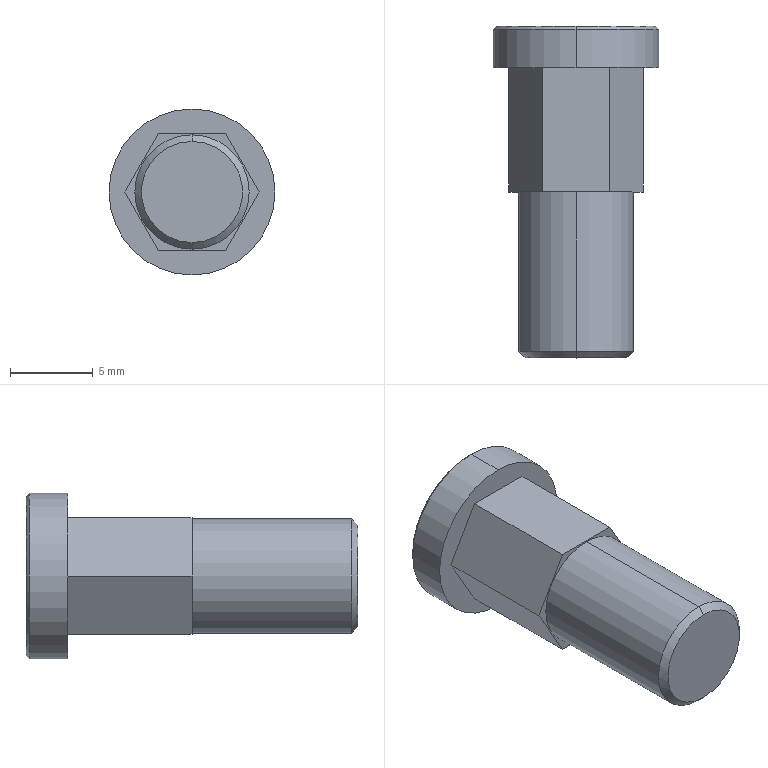Part | NX | features BREP 1 | 1 solid | 24 faces | box 10 x 20 x 10 mm | volume 454.713 mm3 | plane 12 | cylinder 8 | cone 4 | commonest cylinder face diameters 5 x2 6.2 x2 6.9 x2 10 x2
STEP:
#1=CARTESIAN_POINT('',(0.,-10.,-3.45));
#2=VERTEX_POINT('',#1);
#3=CARTESIAN_POINT('',(0.,-10.,3.45));
#4=VERTEX_POINT('',#3);
#5=CARTESIAN_POINT('',(0.,-10.,0.));
#6=DIRECTION('',(0.,-1.,0.));
#7=DIRECTION('',(0.,0.,-1.));
#8=AXIS2_PLACEMENT_3D('',#5,#6,#7);
#9=CIRCLE('',#8,3.45);
#10=EDGE_CURVE('',#2,#4,#9,.T.);
#11=ORIENTED_EDGE('',*,*,#10,.T.);
#12=CARTESIAN_POINT('',(0.,-19.6,3.45));
#13=VERTEX_POINT('',#12);
#14=CARTESIAN_POINT('',(0.,-20.,3.45));
#15=DIRECTION('',(0.,-1.,0.));
#16=VECTOR('',#15,1000.);
#17=LINE('',#14,#16);
#18=EDGE_CURVE('',#13,#4,#17,.F.);
#19=ORIENTED_EDGE('',*,*,#18,.F.);
#20=CARTESIAN_POINT('',(0.,-19.6,-3.45));
#21=VERTEX_POINT('',#20);
#22=CARTESIAN_POINT('',(0.,-19.6,0.));
#23=DIRECTION('',(0.,1.,0.));
#24=DIRECTION('',(0.,0.,-1.));
#25=AXIS2_PLACEMENT_3D('',#22,#23,#24);
#26=CIRCLE('',#25,3.45);
#27=EDGE_CURVE('',#13,#21,#26,.T.);
#28=ORIENTED_EDGE('',*,*,#27,.T.);
#29=CARTESIAN_POINT('',(0.,-20.,-3.45));
#30=DIRECTION('',(0.,-1.,0.));
#31=VECTOR('',#30,1000.);
#32=LINE('',#29,#31);
#33=EDGE_CURVE('',#21,#2,#32,.F.);
#34=ORIENTED_EDGE('',*,*,#33,.T.);
#35=EDGE_LOOP('',(#11,#19,#28,#34));
#36=FACE_BOUND('',#35,.T.);
#37=CARTESIAN_POINT('',(0.,-20.,0.));
#38=DIRECTION('',(0.,-1.,0.));
#39=DIRECTION('',(0.,0.,1.));
#40=AXIS2_PLACEMENT_3D('',#37,#38,#39);
#41=CYLINDRICAL_SURFACE('',#40,3.45);
#42=ADVANCED_FACE('',(#36),#41,.T.);
#43=CARTESIAN_POINT('',(0.,-20.,3.05));
#44=VERTEX_POINT('',#43);
#45=CARTESIAN_POINT('',(0.,-20.,-3.05));
#46=VERTEX_POINT('',#45);
#47=CARTESIAN_POINT('',(0.,-20.,0.));
#48=DIRECTION('',(0.,1.,0.));
#49=DIRECTION('',(0.,0.,1.));
#50=AXIS2_PLACEMENT_3D('',#47,#48,#49);
#51=CIRCLE('',#50,3.05);
#52=EDGE_CURVE('',#44,#46,#51,.T.);
#53=ORIENTED_EDGE('',*,*,#52,.T.);
#54=CARTESIAN_POINT('',(0.,-19.6,-3.45));
#55=DIRECTION('',(0.,0.7071,-0.7071));
#56=VECTOR('',#55,1000.);
#57=LINE('',#54,#56);
#58=EDGE_CURVE('',#46,#21,#57,.T.);
#59=ORIENTED_EDGE('',*,*,#58,.T.);
#60=ORIENTED_EDGE('',*,*,#27,.F.);
#61=CARTESIAN_POINT('',(0.,-19.6,3.45));
#62=DIRECTION('',(0.,0.7071,0.7071));
#63=VECTOR('',#62,1000.);
#64=LINE('',#61,#63);
#65=EDGE_CURVE('',#44,#13,#64,.T.);
#66=ORIENTED_EDGE('',*,*,#65,.F.);
#67=EDGE_LOOP('',(#53,#59,#60,#66));
#68=FACE_BOUND('',#67,.T.);
#69=CARTESIAN_POINT('',(0.,-19.6,0.));
#70=DIRECTION('',(0.,1.,0.));
#71=DIRECTION('',(0.,0.,-1.));
#72=AXIS2_PLACEMENT_3D('',#69,#70,#71);
#73=CONICAL_SURFACE('',#72,3.45,0.7854);
#74=ADVANCED_FACE('',(#68),#73,.T.);
#75=CARTESIAN_POINT('',(0.,-2.5,5.));
#76=VERTEX_POINT('',#75);
#77=CARTESIAN_POINT('',(0.,-2.5,-5.));
#78=VERTEX_POINT('',#77);
#79=CARTESIAN_POINT('',(0.,-2.5,0.));
#80=DIRECTION('',(0.,1.,0.));
#81=DIRECTION('',(0.,0.,1.));
#82=AXIS2_PLACEMENT_3D('',#79,#80,#81);
#83=CIRCLE('',#82,5.);
#84=EDGE_CURVE('',#76,#78,#83,.T.);
#85=ORIENTED_EDGE('',*,*,#84,.T.);
#86=CARTESIAN_POINT('',(0.,-0.2,-5.));
#87=VERTEX_POINT('',#86);
#88=CARTESIAN_POINT('',(0.,0.,-5.));
#89=DIRECTION('',(0.,1.,0.));
#90=VECTOR('',#89,1000.);
#91=LINE('',#88,#90);
#92=EDGE_CURVE('',#78,#87,#91,.T.);
#93=ORIENTED_EDGE('',*,*,#92,.T.);
#94=CARTESIAN_POINT('',(0.,-0.2,5.));
#95=VERTEX_POINT('',#94);
#96=CARTESIAN_POINT('',(0.,-0.2,0.));
#97=DIRECTION('',(0.,-1.,0.));
#98=DIRECTION('',(0.,0.,1.));
#99=AXIS2_PLACEMENT_3D('',#96,#97,#98);
#100=CIRCLE('',#99,5.);
#101=EDGE_CURVE('',#87,#95,#100,.T.);
#102=ORIENTED_EDGE('',*,*,#101,.T.);
#103=CARTESIAN_POINT('',(0.,0.,5.));
#104=DIRECTION('',(0.,1.,0.));
#105=VECTOR('',#104,1000.);
#106=LINE('',#103,#105);
#107=EDGE_CURVE('',#76,#95,#106,.T.);
#108=ORIENTED_EDGE('',*,*,#107,.F.);
#109=EDGE_LOOP('',(#85,#93,#102,#108));
#110=FACE_BOUND('',#109,.T.);
#111=CARTESIAN_POINT('',(0.,0.,0.));
#112=DIRECTION('',(0.,1.,0.));
#113=DIRECTION('',(0.,0.,-1.));
#114=AXIS2_PLACEMENT_3D('',#111,#112,#113);
#115=CYLINDRICAL_SURFACE('',#114,5.);
#116=ADVANCED_FACE('',(#110),#115,.T.);
#117=CARTESIAN_POINT('',(0.,0.,-4.8));
#118=VERTEX_POINT('',#117);
#119=CARTESIAN_POINT('',(0.,0.,4.8));
#120=VERTEX_POINT('',#119);
#121=CARTESIAN_POINT('',(0.,0.,0.));
#122=DIRECTION('',(0.,-1.,0.));
#123=DIRECTION('',(0.,0.,-1.));
#124=AXIS2_PLACEMENT_3D('',#121,#122,#123);
#125=CIRCLE('',#124,4.8);
#126=EDGE_CURVE('',#118,#120,#125,.T.);
#127=ORIENTED_EDGE('',*,*,#126,.T.);
#128=CARTESIAN_POINT('',(0.,-0.2,5.));
#129=DIRECTION('',(0.,-0.7071,0.7071));
#130=VECTOR('',#129,1000.);
#131=LINE('',#128,#130);
#132=EDGE_CURVE('',#95,#120,#131,.F.);
#133=ORIENTED_EDGE('',*,*,#132,.F.);
#134=ORIENTED_EDGE('',*,*,#101,.F.);
#135=CARTESIAN_POINT('',(0.,-0.2,-5.));
#136=DIRECTION('',(0.,-0.7071,-0.7071));
#137=VECTOR('',#136,1000.);
#138=LINE('',#135,#137);
#139=EDGE_CURVE('',#87,#118,#138,.F.);
#140=ORIENTED_EDGE('',*,*,#139,.T.);
#141=EDGE_LOOP('',(#127,#133,#134,#140));
#142=FACE_BOUND('',#141,.T.);
#143=CARTESIAN_POINT('',(0.,-0.2,0.));
#144=DIRECTION('',(0.,-1.,0.));
#145=DIRECTION('',(0.,0.,1.));
#146=AXIS2_PLACEMENT_3D('',#143,#144,#145);
#147=CONICAL_SURFACE('',#146,5.,0.7854);
#148=ADVANCED_FACE('',(#142),#147,.T.);
#149=CARTESIAN_POINT('',(0.,-7.4,-3.1));
#150=VERTEX_POINT('',#149);
#151=CARTESIAN_POINT('',(0.,-7.4,3.1));
#152=VERTEX_POINT('',#151);
#153=CARTESIAN_POINT('',(0.,-7.4,0.));
#154=DIRECTION('',(0.,1.,0.));
#155=DIRECTION('',(0.,0.,1.));
#156=AXIS2_PLACEMENT_3D('',#153,#154,#155);
#157=CIRCLE('',#156,3.1);
#158=EDGE_CURVE('',#150,#152,#157,.T.);
#159=ORIENTED_EDGE('',*,*,#158,.F.);
#160=CARTESIAN_POINT('',(0.,0.,-3.1));
#161=VERTEX_POINT('',#160);
#162=CARTESIAN_POINT('',(0.,0.,-3.1));
#163=DIRECTION('',(0.,1.,0.));
#164=VECTOR('',#163,1000.);
#165=LINE('',#162,#164);
#166=EDGE_CURVE('',#150,#161,#165,.T.);
#167=ORIENTED_EDGE('',*,*,#166,.T.);
#168=CARTESIAN_POINT('',(0.,0.,3.1));
#169=VERTEX_POINT('',#168);
#170=CARTESIAN_POINT('',(0.,0.,0.));
#171=DIRECTION('',(0.,-1.,0.));
#172=DIRECTION('',(0.,0.,1.));
#173=AXIS2_PLACEMENT_3D('',#170,#171,#172);
#174=CIRCLE('',#173,3.1);
#175=EDGE_CURVE('',#169,#161,#174,.T.);
#176=ORIENTED_EDGE('',*,*,#175,.F.);
#177=CARTESIAN_POINT('',(0.,0.,3.1));
#178=DIRECTION('',(0.,1.,0.));
#179=VECTOR('',#178,1000.);
#180=LINE('',#177,#179);
#181=EDGE_CURVE('',#152,#169,#180,.T.);
#182=ORIENTED_EDGE('',*,*,#181,.F.);
#183=EDGE_LOOP('',(#159,#167,#176,#182));
#184=FACE_BOUND('',#183,.T.);
#185=CARTESIAN_POINT('',(0.,0.,0.));
#186=DIRECTION('',(0.,1.,0.));
#187=DIRECTION('',(0.,0.,-1.));
#188=AXIS2_PLACEMENT_3D('',#185,#186,#187);
#189=CYLINDRICAL_SURFACE('',#188,3.1);
#190=ADVANCED_FACE('',(#184),#189,.F.);
#191=CARTESIAN_POINT('',(0.,-18.,-2.5));
#192=VERTEX_POINT('',#191);
#193=CARTESIAN_POINT('',(0.,-18.,2.5));
#194=VERTEX_POINT('',#193);
#195=CARTESIAN_POINT('',(0.,-18.,0.));
#196=DIRECTION('',(0.,1.,0.));
#197=DIRECTION('',(0.,0.,1.));
#198=AXIS2_PLACEMENT_3D('',#195,#196,#197);
#199=CIRCLE('',#198,2.5);
#200=EDGE_CURVE('',#192,#194,#199,.T.);
#201=ORIENTED_EDGE('',*,*,#200,.F.);
#202=CARTESIAN_POINT('',(0.,-7.4,-2.5));
#203=VERTEX_POINT('',#202);
#204=CARTESIAN_POINT('',(0.,-7.4,-2.5));
#205=DIRECTION('',(0.,1.,0.));
#206=VECTOR('',#205,1000.);
#207=LINE('',#204,#206);
#208=EDGE_CURVE('',#192,#203,#207,.T.);
#209=ORIENTED_EDGE('',*,*,#208,.T.);
#210=CARTESIAN_POINT('',(0.,-7.4,2.5));
#211=VERTEX_POINT('',#210);
#212=CARTESIAN_POINT('',(0.,-7.4,0.));
#213=DIRECTION('',(0.,-1.,0.));
#214=DIRECTION('',(0.,0.,1.));
#215=AXIS2_PLACEMENT_3D('',#212,#213,#214);
#216=CIRCLE('',#215,2.5);
#217=EDGE_CURVE('',#211,#203,#216,.T.);
#218=ORIENTED_EDGE('',*,*,#217,.F.);
#219=CARTESIAN_POINT('',(0.,-7.4,2.5));
#220=DIRECTION('',(0.,1.,0.));
#221=VECTOR('',#220,1000.);
#222=LINE('',#219,#221);
#223=EDGE_CURVE('',#194,#211,#222,.T.);
#224=ORIENTED_EDGE('',*,*,#223,.F.);
#225=EDGE_LOOP('',(#201,#209,#218,#224));
#226=FACE_BOUND('',#225,.T.);
#227=CARTESIAN_POINT('',(0.,-7.4,0.));
#228=DIRECTION('',(0.,1.,0.));
#229=DIRECTION('',(0.,0.,-1.));
#230=AXIS2_PLACEMENT_3D('',#227,#228,#229);
#231=CYLINDRICAL_SURFACE('',#230,2.5);
#232=ADVANCED_FACE('',(#226),#231,.F.);
#233=ORIENTED_EDGE('',*,*,#18,.T.);
#234=CARTESIAN_POINT('',(0.,-10.,0.));
#235=DIRECTION('',(0.,-1.,0.));
#236=DIRECTION('',(0.,0.,-1.));
#237=AXIS2_PLACEMENT_3D('',#234,#235,#236);
#238=CIRCLE('',#237,3.45);
#239=EDGE_CURVE('',#4,#2,#238,.T.);
#240=ORIENTED_EDGE('',*,*,#239,.T.);
#241=ORIENTED_EDGE('',*,*,#33,.F.);
#242=CARTESIAN_POINT('',(0.,-19.6,0.));
#243=DIRECTION('',(0.,1.,0.));
#244=DIRECTION('',(0.,0.,-1.));
#245=AXIS2_PLACEMENT_3D('',#242,#243,#244);
#246=CIRCLE('',#245,3.45);
#247=EDGE_CURVE('',#21,#13,#246,.T.);
#248=ORIENTED_EDGE('',*,*,#247,.T.);
#249=EDGE_LOOP('',(#233,#240,#241,#248));
#250=FACE_BOUND('',#249,.T.);
#251=CARTESIAN_POINT('',(0.,-20.,0.));
#252=DIRECTION('',(0.,-1.,0.));
#253=DIRECTION('',(0.,0.,1.));
#254=AXIS2_PLACEMENT_3D('',#251,#252,#253);
#255=CYLINDRICAL_SURFACE('',#254,3.45);
#256=ADVANCED_FACE('',(#250),#255,.T.);
#257=ORIENTED_EDGE('',*,*,#58,.F.);
#258=CARTESIAN_POINT('',(0.,-20.,0.));
#259=DIRECTION('',(0.,1.,0.));
#260=DIRECTION('',(0.,0.,1.));
#261=AXIS2_PLACEMENT_3D('',#258,#259,#260);
#262=CIRCLE('',#261,3.05);
#263=EDGE_CURVE('',#46,#44,#262,.T.);
#264=ORIENTED_EDGE('',*,*,#263,.T.);
#265=ORIENTED_EDGE('',*,*,#65,.T.);
#266=ORIENTED_EDGE('',*,*,#247,.F.);
#267=EDGE_LOOP('',(#257,#264,#265,#266));
#268=FACE_BOUND('',#267,.T.);
#269=CARTESIAN_POINT('',(0.,-19.6,0.));
#270=DIRECTION('',(0.,1.,0.));
#271=DIRECTION('',(0.,0.,-1.));
#272=AXIS2_PLACEMENT_3D('',#269,#270,#271);
#273=CONICAL_SURFACE('',#272,3.45,0.7854);
#274=ADVANCED_FACE('',(#268),#273,.T.);
#275=CARTESIAN_POINT('',(-2.021,-10.,-3.5));
#276=VERTEX_POINT('',#275);
#277=CARTESIAN_POINT('',(2.021,-10.,-3.5));
#278=VERTEX_POINT('',#277);
#279=CARTESIAN_POINT('',(0.,-10.,-3.5));
#280=DIRECTION('',(1.,0.,0.));
#281=VECTOR('',#280,1000.);
#282=LINE('',#279,#281);
#283=EDGE_CURVE('',#276,#278,#282,.T.);
#284=ORIENTED_EDGE('',*,*,#283,.T.);
#285=CARTESIAN_POINT('',(4.041,-10.,0.));
#286=VERTEX_POINT('',#285);
#287=CARTESIAN_POINT('',(2.021,-10.,-3.5));
#288=DIRECTION('',(0.5,0.,0.866));
#289=VECTOR('',#288,1000.);
#290=LINE('',#287,#289);
#291=EDGE_CURVE('',#278,#286,#290,.T.);
#292=ORIENTED_EDGE('',*,*,#291,.T.);
#293=CARTESIAN_POINT('',(2.021,-10.,3.5));
#294=VERTEX_POINT('',#293);
#295=CARTESIAN_POINT('',(4.041,-10.,0.));
#296=DIRECTION('',(-0.5,0.,0.866));
#297=VECTOR('',#296,1000.);
#298=LINE('',#295,#297);
#299=EDGE_CURVE('',#286,#294,#298,.T.);
#300=ORIENTED_EDGE('',*,*,#299,.T.);
#301=CARTESIAN_POINT('',(-2.021,-10.,3.5));
#302=VERTEX_POINT('',#301);
#303=CARTESIAN_POINT('',(0.,-10.,3.5));
#304=DIRECTION('',(-1.,0.,0.));
#305=VECTOR('',#304,1000.);
#306=LINE('',#303,#305);
#307=EDGE_CURVE('',#294,#302,#306,.T.);
#308=ORIENTED_EDGE('',*,*,#307,.T.);
#309=CARTESIAN_POINT('',(-4.041,-10.,0.));
#310=VERTEX_POINT('',#309);
#311=CARTESIAN_POINT('',(-2.021,-10.,3.5));
#312=DIRECTION('',(-0.5,0.,-0.866));
#313=VECTOR('',#312,1000.);
#314=LINE('',#311,#313);
#315=EDGE_CURVE('',#302,#310,#314,.T.);
#316=ORIENTED_EDGE('',*,*,#315,.T.);
#317=CARTESIAN_POINT('',(-4.041,-10.,0.));
#318=DIRECTION('',(0.5,0.,-0.866));
#319=VECTOR('',#318,1000.);
#320=LINE('',#317,#319);
#321=EDGE_CURVE('',#310,#276,#320,.T.);
#322=ORIENTED_EDGE('',*,*,#321,.T.);
#323=EDGE_LOOP('',(#284,#292,#300,#308,#316,#322));
#324=FACE_BOUND('',#323,.T.);
#325=ORIENTED_EDGE('',*,*,#10,.F.);
#326=ORIENTED_EDGE('',*,*,#239,.F.);
#327=EDGE_LOOP('',(#325,#326));
#328=FACE_BOUND('',#327,.T.);
#329=CARTESIAN_POINT('',(0.,-10.,0.));
#330=DIRECTION('',(0.,-1.,0.));
#331=DIRECTION('',(0.,0.,1.));
#332=AXIS2_PLACEMENT_3D('',#329,#330,#331);
#333=PLANE('',#332);
#334=ADVANCED_FACE('',(#324,#328),#333,.T.);
#335=ORIENTED_EDGE('',*,*,#52,.F.);
#336=ORIENTED_EDGE('',*,*,#263,.F.);
#337=EDGE_LOOP('',(#335,#336));
#338=FACE_BOUND('',#337,.T.);
#339=CARTESIAN_POINT('',(0.,-20.,0.));
#340=DIRECTION('',(0.,-1.,0.));
#341=DIRECTION('',(0.,0.,1.));
#342=AXIS2_PLACEMENT_3D('',#339,#340,#341);
#343=PLANE('',#342);
#344=ADVANCED_FACE('',(#338),#343,.T.);
#345=CARTESIAN_POINT('',(2.021,-2.5,-3.5));
#346=VERTEX_POINT('',#345);
#347=CARTESIAN_POINT('',(2.021,-2.5,-3.5));
#348=DIRECTION('',(0.,1.,0.));
#349=VECTOR('',#348,1000.);
#350=LINE('',#347,#349);
#351=EDGE_CURVE('',#278,#346,#350,.T.);
#352=ORIENTED_EDGE('',*,*,#351,.T.);
#353=CARTESIAN_POINT('',(4.041,-2.5,0.));
#354=VERTEX_POINT('',#353);
#355=CARTESIAN_POINT('',(2.021,-2.5,-3.5));
#356=DIRECTION('',(0.5,0.,0.866));
#357=VECTOR('',#356,1000.);
#358=LINE('',#355,#357);
#359=EDGE_CURVE('',#346,#354,#358,.T.);
#360=ORIENTED_EDGE('',*,*,#359,.T.);
#361=CARTESIAN_POINT('',(4.041,-2.5,0.));
#362=DIRECTION('',(0.,-1.,0.));
#363=VECTOR('',#362,1000.);
#364=LINE('',#361,#363);
#365=EDGE_CURVE('',#354,#286,#364,.T.);
#366=ORIENTED_EDGE('',*,*,#365,.T.);
#367=ORIENTED_EDGE('',*,*,#291,.F.);
#368=EDGE_LOOP('',(#352,#360,#366,#367));
#369=FACE_BOUND('',#368,.T.);
#370=CARTESIAN_POINT('',(2.021,-2.5,-3.5));
#371=DIRECTION('',(0.866,0.,-0.5));
#372=DIRECTION('',(0.5,0.,0.866));
#373=AXIS2_PLACEMENT_3D('',#370,#371,#372);
#374=PLANE('',#373);
#375=ADVANCED_FACE('',(#369),#374,.T.);
#376=CARTESIAN_POINT('',(-2.021,-2.5,-3.5));
#377=VERTEX_POINT('',#376);
#378=CARTESIAN_POINT('',(-2.021,-2.5,-3.5));
#379=DIRECTION('',(0.,1.,0.));
#380=VECTOR('',#379,1000.);
#381=LINE('',#378,#380);
#382=EDGE_CURVE('',#276,#377,#381,.T.);
#383=ORIENTED_EDGE('',*,*,#382,.T.);
#384=CARTESIAN_POINT('',(-2.021,-2.5,-3.5));
#385=DIRECTION('',(1.,0.,0.));
#386=VECTOR('',#385,1000.);
#387=LINE('',#384,#386);
#388=EDGE_CURVE('',#377,#346,#387,.T.);
#389=ORIENTED_EDGE('',*,*,#388,.T.);
#390=ORIENTED_EDGE('',*,*,#351,.F.);
#391=ORIENTED_EDGE('',*,*,#283,.F.);
#392=EDGE_LOOP('',(#383,#389,#390,#391));
#393=FACE_BOUND('',#392,.T.);
#394=CARTESIAN_POINT('',(-2.021,-2.5,-3.5));
#395=DIRECTION('',(0.,0.,-1.));
#396=DIRECTION('',(1.,0.,0.));
#397=AXIS2_PLACEMENT_3D('',#394,#395,#396);
#398=PLANE('',#397);
#399=ADVANCED_FACE('',(#393),#398,.T.);
#400=CARTESIAN_POINT('',(-4.041,-2.5,0.));
#401=VERTEX_POINT('',#400);
#402=CARTESIAN_POINT('',(-4.041,-2.5,0.));
#403=DIRECTION('',(0.,1.,0.));
#404=VECTOR('',#403,1000.);
#405=LINE('',#402,#404);
#406=EDGE_CURVE('',#310,#401,#405,.T.);
#407=ORIENTED_EDGE('',*,*,#406,.T.);
#408=CARTESIAN_POINT('',(-4.041,-2.5,0.));
#409=DIRECTION('',(0.5,0.,-0.866));
#410=VECTOR('',#409,1000.);
#411=LINE('',#408,#410);
#412=EDGE_CURVE('',#401,#377,#411,.T.);
#413=ORIENTED_EDGE('',*,*,#412,.T.);
#414=ORIENTED_EDGE('',*,*,#382,.F.);
#415=ORIENTED_EDGE('',*,*,#321,.F.);
#416=EDGE_LOOP('',(#407,#413,#414,#415));
#417=FACE_BOUND('',#416,.T.);
#418=CARTESIAN_POINT('',(-4.041,-2.5,0.));
#419=DIRECTION('',(-0.866,0.,-0.5));
#420=DIRECTION('',(0.5,0.,-0.866));
#421=AXIS2_PLACEMENT_3D('',#418,#419,#420);
#422=PLANE('',#421);
#423=ADVANCED_FACE('',(#417),#422,.T.);
#424=CARTESIAN_POINT('',(-2.021,-2.5,3.5));
#425=VERTEX_POINT('',#424);
#426=CARTESIAN_POINT('',(-2.021,-2.5,3.5));
#427=DIRECTION('',(0.,1.,0.));
#428=VECTOR('',#427,1000.);
#429=LINE('',#426,#428);
#430=EDGE_CURVE('',#302,#425,#429,.T.);
#431=ORIENTED_EDGE('',*,*,#430,.T.);
#432=CARTESIAN_POINT('',(-2.021,-2.5,3.5));
#433=DIRECTION('',(-0.5,0.,-0.866));
#434=VECTOR('',#433,1000.);
#435=LINE('',#432,#434);
#436=EDGE_CURVE('',#425,#401,#435,.T.);
#437=ORIENTED_EDGE('',*,*,#436,.T.);
#438=ORIENTED_EDGE('',*,*,#406,.F.);
#439=ORIENTED_EDGE('',*,*,#315,.F.);
#440=EDGE_LOOP('',(#431,#437,#438,#439));
#441=FACE_BOUND('',#440,.T.);
#442=CARTESIAN_POINT('',(-2.021,-2.5,3.5));
#443=DIRECTION('',(-0.866,0.,0.5));
#444=DIRECTION('',(-0.5,0.,-0.866));
#445=AXIS2_PLACEMENT_3D('',#442,#443,#444);
#446=PLANE('',#445);
#447=ADVANCED_FACE('',(#441),#446,.T.);
#448=CARTESIAN_POINT('',(2.021,-2.5,3.5));
#449=VERTEX_POINT('',#448);
#450=CARTESIAN_POINT('',(2.021,-2.5,3.5));
#451=DIRECTION('',(0.,1.,0.));
#452=VECTOR('',#451,1000.);
#453=LINE('',#450,#452);
#454=EDGE_CURVE('',#294,#449,#453,.T.);
#455=ORIENTED_EDGE('',*,*,#454,.T.);
#456=CARTESIAN_POINT('',(2.021,-2.5,3.5));
#457=DIRECTION('',(-1.,0.,0.));
#458=VECTOR('',#457,1000.);
#459=LINE('',#456,#458);
#460=EDGE_CURVE('',#449,#425,#459,.T.);
#461=ORIENTED_EDGE('',*,*,#460,.T.);
#462=ORIENTED_EDGE('',*,*,#430,.F.);
#463=ORIENTED_EDGE('',*,*,#307,.F.);
#464=EDGE_LOOP('',(#455,#461,#462,#463));
#465=FACE_BOUND('',#464,.T.);
#466=CARTESIAN_POINT('',(2.021,-2.5,3.5));
#467=DIRECTION('',(0.,0.,1.));
#468=DIRECTION('',(-1.,0.,0.));
#469=AXIS2_PLACEMENT_3D('',#466,#467,#468);
#470=PLANE('',#469);
#471=ADVANCED_FACE('',(#465),#470,.T.);
#472=ORIENTED_EDGE('',*,*,#365,.F.);
#473=CARTESIAN_POINT('',(4.041,-2.5,0.));
#474=DIRECTION('',(-0.5,0.,0.866));
#475=VECTOR('',#474,1000.);
#476=LINE('',#473,#475);
#477=EDGE_CURVE('',#354,#449,#476,.T.);
#478=ORIENTED_EDGE('',*,*,#477,.T.);
#479=ORIENTED_EDGE('',*,*,#454,.F.);
#480=ORIENTED_EDGE('',*,*,#299,.F.);
#481=EDGE_LOOP('',(#472,#478,#479,#480));
#482=FACE_BOUND('',#481,.T.);
#483=CARTESIAN_POINT('',(4.041,-2.5,0.));
#484=DIRECTION('',(0.866,0.,0.5));
#485=DIRECTION('',(-0.5,0.,0.866));
#486=AXIS2_PLACEMENT_3D('',#483,#484,#485);
#487=PLANE('',#486);
#488=ADVANCED_FACE('',(#482),#487,.T.);
#489=ORIENTED_EDGE('',*,*,#84,.F.);
#490=CARTESIAN_POINT('',(0.,-2.5,0.));
#491=DIRECTION('',(0.,1.,0.));
#492=DIRECTION('',(0.,0.,1.));
#493=AXIS2_PLACEMENT_3D('',#490,#491,#492);
#494=CIRCLE('',#493,5.);
#495=EDGE_CURVE('',#78,#76,#494,.T.);
#496=ORIENTED_EDGE('',*,*,#495,.F.);
#497=EDGE_LOOP('',(#489,#496));
#498=FACE_BOUND('',#497,.T.);
#499=ORIENTED_EDGE('',*,*,#388,.F.);
#500=ORIENTED_EDGE('',*,*,#412,.F.);
#501=ORIENTED_EDGE('',*,*,#436,.F.);
#502=ORIENTED_EDGE('',*,*,#460,.F.);
#503=ORIENTED_EDGE('',*,*,#477,.F.);
#504=ORIENTED_EDGE('',*,*,#359,.F.);
#505=EDGE_LOOP('',(#499,#500,#501,#502,#503,#504));
#506=FACE_BOUND('',#505,.T.);
#507=CARTESIAN_POINT('',(0.,-2.5,0.));
#508=DIRECTION('',(0.,1.,0.));
#509=DIRECTION('',(0.,0.,-1.));
#510=AXIS2_PLACEMENT_3D('',#507,#508,#509);
#511=PLANE('',#510);
#512=ADVANCED_FACE('',(#498,#506),#511,.F.);
#513=ORIENTED_EDGE('',*,*,#92,.F.);
#514=ORIENTED_EDGE('',*,*,#495,.T.);
#515=ORIENTED_EDGE('',*,*,#107,.T.);
#516=CARTESIAN_POINT('',(0.,-0.2,0.));
#517=DIRECTION('',(0.,-1.,0.));
#518=DIRECTION('',(0.,0.,1.));
#519=AXIS2_PLACEMENT_3D('',#516,#517,#518);
#520=CIRCLE('',#519,5.);
#521=EDGE_CURVE('',#95,#87,#520,.T.);
#522=ORIENTED_EDGE('',*,*,#521,.T.);
#523=EDGE_LOOP('',(#513,#514,#515,#522));
#524=FACE_BOUND('',#523,.T.);
#525=CARTESIAN_POINT('',(0.,0.,0.));
#526=DIRECTION('',(0.,1.,0.));
#527=DIRECTION('',(0.,0.,-1.));
#528=AXIS2_PLACEMENT_3D('',#525,#526,#527);
#529=CYLINDRICAL_SURFACE('',#528,5.);
#530=ADVANCED_FACE('',(#524),#529,.T.);
#531=ORIENTED_EDGE('',*,*,#132,.T.);
#532=CARTESIAN_POINT('',(0.,0.,0.));
#533=DIRECTION('',(0.,-1.,0.));
#534=DIRECTION('',(0.,0.,-1.));
#535=AXIS2_PLACEMENT_3D('',#532,#533,#534);
#536=CIRCLE('',#535,4.8);
#537=EDGE_CURVE('',#120,#118,#536,.T.);
#538=ORIENTED_EDGE('',*,*,#537,.T.);
#539=ORIENTED_EDGE('',*,*,#139,.F.);
#540=ORIENTED_EDGE('',*,*,#521,.F.);
#541=EDGE_LOOP('',(#531,#538,#539,#540));
#542=FACE_BOUND('',#541,.T.);
#543=CARTESIAN_POINT('',(0.,-0.2,0.));
#544=DIRECTION('',(0.,-1.,0.));
#545=DIRECTION('',(0.,0.,1.));
#546=AXIS2_PLACEMENT_3D('',#543,#544,#545);
#547=CONICAL_SURFACE('',#546,5.,0.7854);
#548=ADVANCED_FACE('',(#542),#547,.T.);
#549=ORIENTED_EDGE('',*,*,#126,.F.);
#550=ORIENTED_EDGE('',*,*,#537,.F.);
#551=EDGE_LOOP('',(#549,#550));
#552=FACE_BOUND('',#551,.T.);
#553=ORIENTED_EDGE('',*,*,#175,.T.);
#554=CARTESIAN_POINT('',(0.,0.,0.));
#555=DIRECTION('',(0.,-1.,0.));
#556=DIRECTION('',(0.,0.,1.));
#557=AXIS2_PLACEMENT_3D('',#554,#555,#556);
#558=CIRCLE('',#557,3.1);
#559=EDGE_CURVE('',#161,#169,#558,.T.);
#560=ORIENTED_EDGE('',*,*,#559,.T.);
#561=EDGE_LOOP('',(#553,#560));
#562=FACE_BOUND('',#561,.T.);
#563=CARTESIAN_POINT('',(0.,0.,0.));
#564=DIRECTION('',(0.,1.,0.));
#565=DIRECTION('',(0.,0.,-1.));
#566=AXIS2_PLACEMENT_3D('',#563,#564,#565);
#567=PLANE('',#566);
#568=ADVANCED_FACE('',(#552,#562),#567,.T.);
#569=ORIENTED_EDGE('',*,*,#166,.F.);
#570=CARTESIAN_POINT('',(0.,-7.4,0.));
#571=DIRECTION('',(0.,1.,0.));
#572=DIRECTION('',(0.,0.,1.));
#573=AXIS2_PLACEMENT_3D('',#570,#571,#572);
#574=CIRCLE('',#573,3.1);
#575=EDGE_CURVE('',#152,#150,#574,.T.);
#576=ORIENTED_EDGE('',*,*,#575,.F.);
#577=ORIENTED_EDGE('',*,*,#181,.T.);
#578=ORIENTED_EDGE('',*,*,#559,.F.);
#579=EDGE_LOOP('',(#569,#576,#577,#578));
#580=FACE_BOUND('',#579,.T.);
#581=CARTESIAN_POINT('',(0.,0.,0.));
#582=DIRECTION('',(0.,1.,0.));
#583=DIRECTION('',(0.,0.,-1.));
#584=AXIS2_PLACEMENT_3D('',#581,#582,#583);
#585=CYLINDRICAL_SURFACE('',#584,3.1);
#586=ADVANCED_FACE('',(#580),#585,.F.);
#587=ORIENTED_EDGE('',*,*,#575,.T.);
#588=ORIENTED_EDGE('',*,*,#158,.T.);
#589=EDGE_LOOP('',(#587,#588));
#590=FACE_BOUND('',#589,.T.);
#591=ORIENTED_EDGE('',*,*,#217,.T.);
#592=CARTESIAN_POINT('',(0.,-7.4,0.));
#593=DIRECTION('',(0.,-1.,0.));
#594=DIRECTION('',(0.,0.,1.));
#595=AXIS2_PLACEMENT_3D('',#592,#593,#594);
#596=CIRCLE('',#595,2.5);
#597=EDGE_CURVE('',#203,#211,#596,.T.);
#598=ORIENTED_EDGE('',*,*,#597,.T.);
#599=EDGE_LOOP('',(#591,#598));
#600=FACE_BOUND('',#599,.T.);
#601=CARTESIAN_POINT('',(0.,-7.4,0.));
#602=DIRECTION('',(0.,1.,0.));
#603=DIRECTION('',(0.,0.,-1.));
#604=AXIS2_PLACEMENT_3D('',#601,#602,#603);
#605=PLANE('',#604);
#606=ADVANCED_FACE('',(#590,#600),#605,.T.);
#607=ORIENTED_EDGE('',*,*,#208,.F.);
#608=CARTESIAN_POINT('',(0.,-18.,0.));
#609=DIRECTION('',(0.,1.,0.));
#610=DIRECTION('',(0.,0.,1.));
#611=AXIS2_PLACEMENT_3D('',#608,#609,#610);
#612=CIRCLE('',#611,2.5);
#613=EDGE_CURVE('',#194,#192,#612,.T.);
#614=ORIENTED_EDGE('',*,*,#613,.F.);
#615=ORIENTED_EDGE('',*,*,#223,.T.);
#616=ORIENTED_EDGE('',*,*,#597,.F.);
#617=EDGE_LOOP('',(#607,#614,#615,#616));
#618=FACE_BOUND('',#617,.T.);
#619=CARTESIAN_POINT('',(0.,-7.4,0.));
#620=DIRECTION('',(0.,1.,0.));
#621=DIRECTION('',(0.,0.,-1.));
#622=AXIS2_PLACEMENT_3D('',#619,#620,#621);
#623=CYLINDRICAL_SURFACE('',#622,2.5);
#624=ADVANCED_FACE('',(#618),#623,.F.);
#625=ORIENTED_EDGE('',*,*,#613,.T.);
#626=ORIENTED_EDGE('',*,*,#200,.T.);
#627=EDGE_LOOP('',(#625,#626));
#628=FACE_BOUND('',#627,.T.);
#629=CARTESIAN_POINT('',(0.,-18.,0.));
#630=DIRECTION('',(0.,1.,0.));
#631=DIRECTION('',(0.,0.,-1.));
#632=AXIS2_PLACEMENT_3D('',#629,#630,#631);
#633=PLANE('',#632);
#634=ADVANCED_FACE('',(#628),#633,.T.);
#635=CLOSED_SHELL('',(#42,#74,#116,#148,#190,#232,#256,#274,#334,#344,#375,#399,#423,#447,#471,#488,#512,#530,#548,#568,#586,#606,#624,#634));
#636=MANIFOLD_SOLID_BREP('',#635);
#637=(LENGTH_UNIT()NAMED_UNIT(*)SI_UNIT(.MILLI.,.METRE.));
#638=UNCERTAINTY_MEASURE_WITH_UNIT(LENGTH_MEASURE(0.00001),#637,'','');
#639=(NAMED_UNIT(*)PLANE_ANGLE_UNIT()SI_UNIT($,.RADIAN.));
#640=(NAMED_UNIT(*)SI_UNIT($,.STERADIAN.)SOLID_ANGLE_UNIT());
#641=(GEOMETRIC_REPRESENTATION_CONTEXT(3)GLOBAL_UNCERTAINTY_ASSIGNED_CONTEXT((#638))GLOBAL_UNIT_ASSIGNED_CONTEXT((#637,#639,#640))REPRESENTATION_CONTEXT('',''));
#642=ADVANCED_BREP_SHAPE_REPRESENTATION('',(#636),#641);